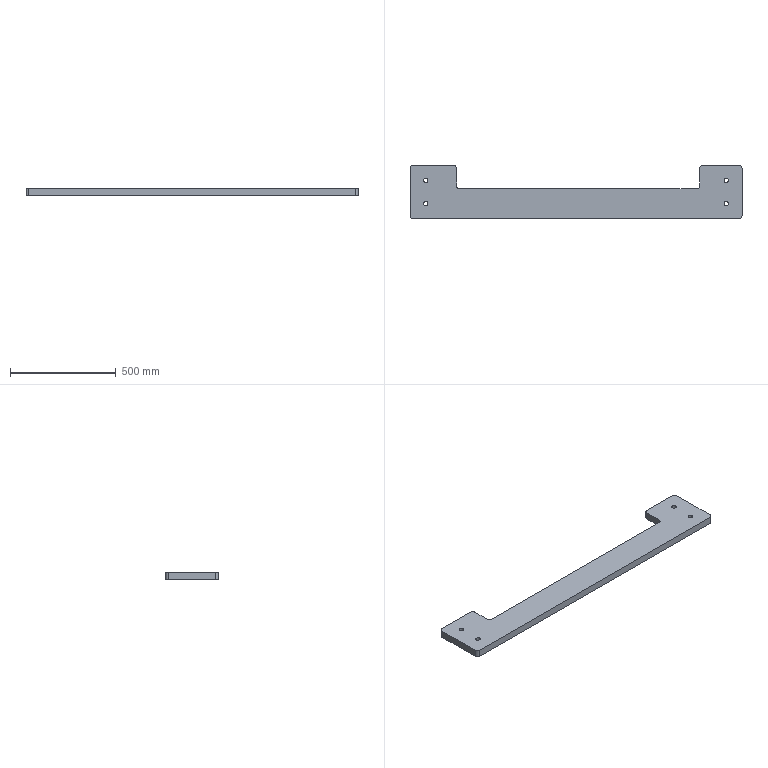Part | SolidWorks | features SavedExtBody 1 | 1 solid | 26 faces | box 1570 x 250 x 35 mm | volume 9261323 mm3 | cylinder 16 | plane 10 | commonest cylinder face diameters 20 x8 25 x8
STEP:
#1=CARTESIAN_POINT('',(-720.,-55.,0.));
#2=VERTEX_POINT('',#1);
#3=CARTESIAN_POINT('',(-700.,-55.,0.));
#4=VERTEX_POINT('',#3);
#5=CARTESIAN_POINT('',(-710.,-55.,0.));
#6=DIRECTION('',(0.,0.,1.));
#7=DIRECTION('',(-1.,0.,0.));
#8=AXIS2_PLACEMENT_3D('',#5,#6,#7);
#9=CIRCLE('',#8,10.);
#10=EDGE_CURVE('',#2,#4,#9,.T.);
#11=ORIENTED_EDGE('',*,*,#10,.F.);
#12=CARTESIAN_POINT('',(-720.,-55.,35.));
#13=VERTEX_POINT('',#12);
#14=CARTESIAN_POINT('',(-720.,-55.,-0.001));
#15=DIRECTION('',(0.,0.,1.));
#16=VECTOR('',#15,1000.);
#17=LINE('',#14,#16);
#18=EDGE_CURVE('',#2,#13,#17,.T.);
#19=ORIENTED_EDGE('',*,*,#18,.T.);
#20=CARTESIAN_POINT('',(-700.,-55.,35.));
#21=VERTEX_POINT('',#20);
#22=CARTESIAN_POINT('',(-710.,-55.,35.));
#23=DIRECTION('',(0.,0.,1.));
#24=DIRECTION('',(1.,0.,0.));
#25=AXIS2_PLACEMENT_3D('',#22,#23,#24);
#26=CIRCLE('',#25,10.);
#27=EDGE_CURVE('',#13,#21,#26,.T.);
#28=ORIENTED_EDGE('',*,*,#27,.T.);
#29=CARTESIAN_POINT('',(-700.,-55.,-0.001));
#30=DIRECTION('',(0.,0.,1.));
#31=VECTOR('',#30,1000.);
#32=LINE('',#29,#31);
#33=EDGE_CURVE('',#4,#21,#32,.T.);
#34=ORIENTED_EDGE('',*,*,#33,.F.);
#35=EDGE_LOOP('',(#11,#19,#28,#34));
#36=FACE_OUTER_BOUND('',#35,.T.);
#37=CARTESIAN_POINT('',(-710.,-55.,-0.001));
#38=DIRECTION('',(0.,0.,1.));
#39=DIRECTION('',(1.,0.,0.));
#40=AXIS2_PLACEMENT_3D('',#37,#38,#39);
#41=CYLINDRICAL_SURFACE('',#40,10.);
#42=ADVANCED_FACE('',(#36),#41,.F.);
#43=CARTESIAN_POINT('',(700.,55.,0.));
#44=VERTEX_POINT('',#43);
#45=CARTESIAN_POINT('',(720.,55.,0.));
#46=VERTEX_POINT('',#45);
#47=CARTESIAN_POINT('',(710.,55.,0.));
#48=DIRECTION('',(0.,0.,1.));
#49=DIRECTION('',(-1.,0.,0.));
#50=AXIS2_PLACEMENT_3D('',#47,#48,#49);
#51=CIRCLE('',#50,10.);
#52=EDGE_CURVE('',#44,#46,#51,.T.);
#53=ORIENTED_EDGE('',*,*,#52,.F.);
#54=CARTESIAN_POINT('',(700.,55.,35.));
#55=VERTEX_POINT('',#54);
#56=CARTESIAN_POINT('',(700.,55.,-0.001));
#57=DIRECTION('',(0.,0.,1.));
#58=VECTOR('',#57,1000.);
#59=LINE('',#56,#58);
#60=EDGE_CURVE('',#44,#55,#59,.T.);
#61=ORIENTED_EDGE('',*,*,#60,.T.);
#62=CARTESIAN_POINT('',(720.,55.,35.));
#63=VERTEX_POINT('',#62);
#64=CARTESIAN_POINT('',(710.,55.,35.));
#65=DIRECTION('',(0.,0.,1.));
#66=DIRECTION('',(1.,0.,0.));
#67=AXIS2_PLACEMENT_3D('',#64,#65,#66);
#68=CIRCLE('',#67,10.);
#69=EDGE_CURVE('',#55,#63,#68,.T.);
#70=ORIENTED_EDGE('',*,*,#69,.T.);
#71=CARTESIAN_POINT('',(720.,55.,-0.001));
#72=DIRECTION('',(0.,0.,1.));
#73=VECTOR('',#72,1000.);
#74=LINE('',#71,#73);
#75=EDGE_CURVE('',#46,#63,#74,.T.);
#76=ORIENTED_EDGE('',*,*,#75,.F.);
#77=EDGE_LOOP('',(#53,#61,#70,#76));
#78=FACE_OUTER_BOUND('',#77,.T.);
#79=CARTESIAN_POINT('',(710.,55.,-0.001));
#80=DIRECTION('',(0.,0.,1.));
#81=DIRECTION('',(1.,0.,0.));
#82=AXIS2_PLACEMENT_3D('',#79,#80,#81);
#83=CYLINDRICAL_SURFACE('',#82,10.);
#84=ADVANCED_FACE('',(#78),#83,.F.);
#85=CARTESIAN_POINT('',(700.,-55.,0.));
#86=VERTEX_POINT('',#85);
#87=CARTESIAN_POINT('',(720.,-55.,0.));
#88=VERTEX_POINT('',#87);
#89=CARTESIAN_POINT('',(710.,-55.,0.));
#90=DIRECTION('',(0.,0.,1.));
#91=DIRECTION('',(-1.,0.,0.));
#92=AXIS2_PLACEMENT_3D('',#89,#90,#91);
#93=CIRCLE('',#92,10.);
#94=EDGE_CURVE('',#86,#88,#93,.T.);
#95=ORIENTED_EDGE('',*,*,#94,.F.);
#96=CARTESIAN_POINT('',(700.,-55.,35.));
#97=VERTEX_POINT('',#96);
#98=CARTESIAN_POINT('',(700.,-55.,-0.001));
#99=DIRECTION('',(0.,0.,1.));
#100=VECTOR('',#99,1000.);
#101=LINE('',#98,#100);
#102=EDGE_CURVE('',#86,#97,#101,.T.);
#103=ORIENTED_EDGE('',*,*,#102,.T.);
#104=CARTESIAN_POINT('',(720.,-55.,35.));
#105=VERTEX_POINT('',#104);
#106=CARTESIAN_POINT('',(710.,-55.,35.));
#107=DIRECTION('',(0.,0.,1.));
#108=DIRECTION('',(1.,0.,0.));
#109=AXIS2_PLACEMENT_3D('',#106,#107,#108);
#110=CIRCLE('',#109,10.);
#111=EDGE_CURVE('',#97,#105,#110,.T.);
#112=ORIENTED_EDGE('',*,*,#111,.T.);
#113=CARTESIAN_POINT('',(720.,-55.,-0.001));
#114=DIRECTION('',(0.,0.,1.));
#115=VECTOR('',#114,1000.);
#116=LINE('',#113,#115);
#117=EDGE_CURVE('',#88,#105,#116,.T.);
#118=ORIENTED_EDGE('',*,*,#117,.F.);
#119=EDGE_LOOP('',(#95,#103,#112,#118));
#120=FACE_OUTER_BOUND('',#119,.T.);
#121=CARTESIAN_POINT('',(710.,-55.,-0.001));
#122=DIRECTION('',(0.,0.,1.));
#123=DIRECTION('',(1.,0.,0.));
#124=AXIS2_PLACEMENT_3D('',#121,#122,#123);
#125=CYLINDRICAL_SURFACE('',#124,10.);
#126=ADVANCED_FACE('',(#120),#125,.F.);
#127=CARTESIAN_POINT('',(-720.,55.,0.));
#128=VERTEX_POINT('',#127);
#129=CARTESIAN_POINT('',(-700.,55.,0.));
#130=VERTEX_POINT('',#129);
#131=CARTESIAN_POINT('',(-710.,55.,0.));
#132=DIRECTION('',(0.,0.,1.));
#133=DIRECTION('',(-1.,0.,0.));
#134=AXIS2_PLACEMENT_3D('',#131,#132,#133);
#135=CIRCLE('',#134,10.);
#136=EDGE_CURVE('',#128,#130,#135,.T.);
#137=ORIENTED_EDGE('',*,*,#136,.F.);
#138=CARTESIAN_POINT('',(-720.,55.,35.));
#139=VERTEX_POINT('',#138);
#140=CARTESIAN_POINT('',(-720.,55.,-0.001));
#141=DIRECTION('',(0.,0.,1.));
#142=VECTOR('',#141,1000.);
#143=LINE('',#140,#142);
#144=EDGE_CURVE('',#128,#139,#143,.T.);
#145=ORIENTED_EDGE('',*,*,#144,.T.);
#146=CARTESIAN_POINT('',(-700.,55.,35.));
#147=VERTEX_POINT('',#146);
#148=CARTESIAN_POINT('',(-710.,55.,35.));
#149=DIRECTION('',(0.,0.,1.));
#150=DIRECTION('',(1.,0.,0.));
#151=AXIS2_PLACEMENT_3D('',#148,#149,#150);
#152=CIRCLE('',#151,10.);
#153=EDGE_CURVE('',#139,#147,#152,.T.);
#154=ORIENTED_EDGE('',*,*,#153,.T.);
#155=CARTESIAN_POINT('',(-700.,55.,-0.001));
#156=DIRECTION('',(0.,0.,1.));
#157=VECTOR('',#156,1000.);
#158=LINE('',#155,#157);
#159=EDGE_CURVE('',#130,#147,#158,.T.);
#160=ORIENTED_EDGE('',*,*,#159,.F.);
#161=EDGE_LOOP('',(#137,#145,#154,#160));
#162=FACE_OUTER_BOUND('',#161,.T.);
#163=CARTESIAN_POINT('',(-710.,55.,-0.001));
#164=DIRECTION('',(0.,0.,1.));
#165=DIRECTION('',(1.,0.,0.));
#166=AXIS2_PLACEMENT_3D('',#163,#164,#165);
#167=CYLINDRICAL_SURFACE('',#166,10.);
#168=ADVANCED_FACE('',(#162),#167,.F.);
#169=CARTESIAN_POINT('',(772.5,125.,0.));
#170=VERTEX_POINT('',#169);
#171=CARTESIAN_POINT('',(597.5,125.,0.));
#172=VERTEX_POINT('',#171);
#173=CARTESIAN_POINT('',(-785.,125.,0.));
#174=DIRECTION('',(-1.,0.,0.));
#175=VECTOR('',#174,1000.);
#176=LINE('',#173,#175);
#177=EDGE_CURVE('',#170,#172,#176,.T.);
#178=ORIENTED_EDGE('',*,*,#177,.T.);
#179=CARTESIAN_POINT('',(597.5,125.,35.));
#180=VERTEX_POINT('',#179);
#181=CARTESIAN_POINT('',(597.5,125.,35.));
#182=DIRECTION('',(0.,0.,1.));
#183=VECTOR('',#182,1000.);
#184=LINE('',#181,#183);
#185=EDGE_CURVE('',#172,#180,#184,.T.);
#186=ORIENTED_EDGE('',*,*,#185,.T.);
#187=CARTESIAN_POINT('',(772.5,125.,35.));
#188=VERTEX_POINT('',#187);
#189=CARTESIAN_POINT('',(-785.,125.,35.));
#190=DIRECTION('',(-1.,0.,0.));
#191=VECTOR('',#190,1000.);
#192=LINE('',#189,#191);
#193=EDGE_CURVE('',#188,#180,#192,.T.);
#194=ORIENTED_EDGE('',*,*,#193,.F.);
#195=CARTESIAN_POINT('',(772.5,125.,35.));
#196=DIRECTION('',(0.,0.,-1.));
#197=VECTOR('',#196,1000.);
#198=LINE('',#195,#197);
#199=EDGE_CURVE('',#188,#170,#198,.T.);
#200=ORIENTED_EDGE('',*,*,#199,.T.);
#201=EDGE_LOOP('',(#178,#186,#194,#200));
#202=FACE_OUTER_BOUND('',#201,.T.);
#203=CARTESIAN_POINT('',(-785.,125.,35.));
#204=DIRECTION('',(0.,-1.,0.));
#205=DIRECTION('',(0.,0.,-1.));
#206=AXIS2_PLACEMENT_3D('',#203,#204,#205);
#207=PLANE('',#206);
#208=ADVANCED_FACE('',(#202),#207,.F.);
#209=CARTESIAN_POINT('',(785.,-112.5,0.));
#210=VERTEX_POINT('',#209);
#211=CARTESIAN_POINT('',(785.,112.5,0.));
#212=VERTEX_POINT('',#211);
#213=CARTESIAN_POINT('',(785.,-125.,0.));
#214=DIRECTION('',(0.,1.,0.));
#215=VECTOR('',#214,1000.);
#216=LINE('',#213,#215);
#217=EDGE_CURVE('',#210,#212,#216,.T.);
#218=ORIENTED_EDGE('',*,*,#217,.T.);
#219=CARTESIAN_POINT('',(785.,112.5,35.));
#220=VERTEX_POINT('',#219);
#221=CARTESIAN_POINT('',(785.,112.5,35.));
#222=DIRECTION('',(0.,0.,1.));
#223=VECTOR('',#222,1000.);
#224=LINE('',#221,#223);
#225=EDGE_CURVE('',#212,#220,#224,.T.);
#226=ORIENTED_EDGE('',*,*,#225,.T.);
#227=CARTESIAN_POINT('',(785.,-112.5,35.));
#228=VERTEX_POINT('',#227);
#229=CARTESIAN_POINT('',(785.,-125.,35.));
#230=DIRECTION('',(0.,1.,0.));
#231=VECTOR('',#230,1000.);
#232=LINE('',#229,#231);
#233=EDGE_CURVE('',#228,#220,#232,.T.);
#234=ORIENTED_EDGE('',*,*,#233,.F.);
#235=CARTESIAN_POINT('',(785.,-112.5,35.));
#236=DIRECTION('',(0.,0.,-1.));
#237=VECTOR('',#236,1000.);
#238=LINE('',#235,#237);
#239=EDGE_CURVE('',#228,#210,#238,.T.);
#240=ORIENTED_EDGE('',*,*,#239,.T.);
#241=EDGE_LOOP('',(#218,#226,#234,#240));
#242=FACE_OUTER_BOUND('',#241,.T.);
#243=CARTESIAN_POINT('',(785.,-125.,35.));
#244=DIRECTION('',(-1.,0.,0.));
#245=DIRECTION('',(0.,0.,1.));
#246=AXIS2_PLACEMENT_3D('',#243,#244,#245);
#247=PLANE('',#246);
#248=ADVANCED_FACE('',(#242),#247,.F.);
#249=CARTESIAN_POINT('',(-577.5,125.,35.));
#250=VERTEX_POINT('',#249);
#251=CARTESIAN_POINT('',(-772.5,125.,35.));
#252=VERTEX_POINT('',#251);
#253=CARTESIAN_POINT('',(-785.,125.,35.));
#254=DIRECTION('',(-1.,0.,0.));
#255=VECTOR('',#254,1000.);
#256=LINE('',#253,#255);
#257=EDGE_CURVE('',#250,#252,#256,.T.);
#258=ORIENTED_EDGE('',*,*,#257,.F.);
#259=CARTESIAN_POINT('',(-577.5,125.,0.));
#260=VERTEX_POINT('',#259);
#261=CARTESIAN_POINT('',(-577.5,125.,35.));
#262=DIRECTION('',(0.,0.,-1.));
#263=VECTOR('',#262,1000.);
#264=LINE('',#261,#263);
#265=EDGE_CURVE('',#250,#260,#264,.T.);
#266=ORIENTED_EDGE('',*,*,#265,.T.);
#267=CARTESIAN_POINT('',(-772.5,125.,0.));
#268=VERTEX_POINT('',#267);
#269=CARTESIAN_POINT('',(-785.,125.,0.));
#270=DIRECTION('',(-1.,0.,0.));
#271=VECTOR('',#270,1000.);
#272=LINE('',#269,#271);
#273=EDGE_CURVE('',#260,#268,#272,.T.);
#274=ORIENTED_EDGE('',*,*,#273,.T.);
#275=CARTESIAN_POINT('',(-772.5,125.,35.));
#276=DIRECTION('',(0.,0.,1.));
#277=VECTOR('',#276,1000.);
#278=LINE('',#275,#277);
#279=EDGE_CURVE('',#268,#252,#278,.T.);
#280=ORIENTED_EDGE('',*,*,#279,.T.);
#281=EDGE_LOOP('',(#258,#266,#274,#280));
#282=FACE_OUTER_BOUND('',#281,.T.);
#283=CARTESIAN_POINT('',(-785.,125.,35.));
#284=DIRECTION('',(0.,-1.,0.));
#285=DIRECTION('',(0.,0.,-1.));
#286=AXIS2_PLACEMENT_3D('',#283,#284,#285);
#287=PLANE('',#286);
#288=ADVANCED_FACE('',(#282),#287,.F.);
#289=CARTESIAN_POINT('',(-785.,112.5,0.));
#290=VERTEX_POINT('',#289);
#291=CARTESIAN_POINT('',(-785.,-112.5,0.));
#292=VERTEX_POINT('',#291);
#293=CARTESIAN_POINT('',(-785.,-125.,0.));
#294=DIRECTION('',(0.,-1.,0.));
#295=VECTOR('',#294,1000.);
#296=LINE('',#293,#295);
#297=EDGE_CURVE('',#290,#292,#296,.T.);
#298=ORIENTED_EDGE('',*,*,#297,.T.);
#299=CARTESIAN_POINT('',(-785.,-112.5,35.));
#300=VERTEX_POINT('',#299);
#301=CARTESIAN_POINT('',(-785.,-112.5,35.));
#302=DIRECTION('',(0.,0.,1.));
#303=VECTOR('',#302,1000.);
#304=LINE('',#301,#303);
#305=EDGE_CURVE('',#292,#300,#304,.T.);
#306=ORIENTED_EDGE('',*,*,#305,.T.);
#307=CARTESIAN_POINT('',(-785.,112.5,35.));
#308=VERTEX_POINT('',#307);
#309=CARTESIAN_POINT('',(-785.,-125.,35.));
#310=DIRECTION('',(0.,-1.,0.));
#311=VECTOR('',#310,1000.);
#312=LINE('',#309,#311);
#313=EDGE_CURVE('',#308,#300,#312,.T.);
#314=ORIENTED_EDGE('',*,*,#313,.F.);
#315=CARTESIAN_POINT('',(-785.,112.5,35.));
#316=DIRECTION('',(0.,0.,-1.));
#317=VECTOR('',#316,1000.);
#318=LINE('',#315,#317);
#319=EDGE_CURVE('',#308,#290,#318,.T.);
#320=ORIENTED_EDGE('',*,*,#319,.T.);
#321=EDGE_LOOP('',(#298,#306,#314,#320));
#322=FACE_OUTER_BOUND('',#321,.T.);
#323=CARTESIAN_POINT('',(-785.,-125.,35.));
#324=DIRECTION('',(1.,0.,0.));
#325=DIRECTION('',(0.,0.,-1.));
#326=AXIS2_PLACEMENT_3D('',#323,#324,#325);
#327=PLANE('',#326);
#328=ADVANCED_FACE('',(#322),#327,.F.);
#329=CARTESIAN_POINT('',(-772.5,-125.,0.));
#330=VERTEX_POINT('',#329);
#331=CARTESIAN_POINT('',(772.5,-125.,0.));
#332=VERTEX_POINT('',#331);
#333=CARTESIAN_POINT('',(-785.,-125.,0.));
#334=DIRECTION('',(1.,0.,0.));
#335=VECTOR('',#334,1000.);
#336=LINE('',#333,#335);
#337=EDGE_CURVE('',#330,#332,#336,.T.);
#338=ORIENTED_EDGE('',*,*,#337,.T.);
#339=CARTESIAN_POINT('',(772.5,-125.,35.));
#340=VERTEX_POINT('',#339);
#341=CARTESIAN_POINT('',(772.5,-125.,35.));
#342=DIRECTION('',(0.,0.,1.));
#343=VECTOR('',#342,1000.);
#344=LINE('',#341,#343);
#345=EDGE_CURVE('',#332,#340,#344,.T.);
#346=ORIENTED_EDGE('',*,*,#345,.T.);
#347=CARTESIAN_POINT('',(-772.5,-125.,35.));
#348=VERTEX_POINT('',#347);
#349=CARTESIAN_POINT('',(-785.,-125.,35.));
#350=DIRECTION('',(1.,0.,0.));
#351=VECTOR('',#350,1000.);
#352=LINE('',#349,#351);
#353=EDGE_CURVE('',#348,#340,#352,.T.);
#354=ORIENTED_EDGE('',*,*,#353,.F.);
#355=CARTESIAN_POINT('',(-772.5,-125.,35.));
#356=DIRECTION('',(0.,0.,-1.));
#357=VECTOR('',#356,1000.);
#358=LINE('',#355,#357);
#359=EDGE_CURVE('',#348,#330,#358,.T.);
#360=ORIENTED_EDGE('',*,*,#359,.T.);
#361=EDGE_LOOP('',(#338,#346,#354,#360));
#362=FACE_OUTER_BOUND('',#361,.T.);
#363=CARTESIAN_POINT('',(-785.,-125.,35.));
#364=DIRECTION('',(0.,1.,0.));
#365=DIRECTION('',(0.,0.,1.));
#366=AXIS2_PLACEMENT_3D('',#363,#364,#365);
#367=PLANE('',#366);
#368=ADVANCED_FACE('',(#362),#367,.F.);
#369=CARTESIAN_POINT('',(-710.,-55.,35.));
#370=DIRECTION('',(0.,0.,1.));
#371=DIRECTION('',(1.,0.,0.));
#372=AXIS2_PLACEMENT_3D('',#369,#370,#371);
#373=CIRCLE('',#372,10.);
#374=EDGE_CURVE('',#21,#13,#373,.T.);
#375=ORIENTED_EDGE('',*,*,#374,.F.);
#376=ORIENTED_EDGE('',*,*,#27,.F.);
#377=EDGE_LOOP('',(#375,#376));
#378=FACE_BOUND('',#377,.T.);
#379=CARTESIAN_POINT('',(710.,55.,35.));
#380=DIRECTION('',(0.,0.,1.));
#381=DIRECTION('',(1.,0.,0.));
#382=AXIS2_PLACEMENT_3D('',#379,#380,#381);
#383=CIRCLE('',#382,10.);
#384=EDGE_CURVE('',#63,#55,#383,.T.);
#385=ORIENTED_EDGE('',*,*,#384,.F.);
#386=ORIENTED_EDGE('',*,*,#69,.F.);
#387=EDGE_LOOP('',(#385,#386));
#388=FACE_BOUND('',#387,.T.);
#389=CARTESIAN_POINT('',(710.,-55.,35.));
#390=DIRECTION('',(0.,0.,1.));
#391=DIRECTION('',(1.,0.,0.));
#392=AXIS2_PLACEMENT_3D('',#389,#390,#391);
#393=CIRCLE('',#392,10.);
#394=EDGE_CURVE('',#105,#97,#393,.T.);
#395=ORIENTED_EDGE('',*,*,#394,.F.);
#396=ORIENTED_EDGE('',*,*,#111,.F.);
#397=EDGE_LOOP('',(#395,#396));
#398=FACE_BOUND('',#397,.T.);
#399=CARTESIAN_POINT('',(-710.,55.,35.));
#400=DIRECTION('',(0.,0.,1.));
#401=DIRECTION('',(1.,0.,0.));
#402=AXIS2_PLACEMENT_3D('',#399,#400,#401);
#403=CIRCLE('',#402,10.);
#404=EDGE_CURVE('',#147,#139,#403,.T.);
#405=ORIENTED_EDGE('',*,*,#404,.F.);
#406=ORIENTED_EDGE('',*,*,#153,.F.);
#407=EDGE_LOOP('',(#405,#406));
#408=FACE_BOUND('',#407,.T.);
#409=CARTESIAN_POINT('',(-565.,112.5,35.));
#410=VERTEX_POINT('',#409);
#411=CARTESIAN_POINT('',(-565.,27.5,35.));
#412=VERTEX_POINT('',#411);
#413=CARTESIAN_POINT('',(-565.,125.,35.));
#414=DIRECTION('',(0.,-1.,0.));
#415=VECTOR('',#414,1000.);
#416=LINE('',#413,#415);
#417=EDGE_CURVE('',#410,#412,#416,.T.);
#418=ORIENTED_EDGE('',*,*,#417,.F.);
#419=CARTESIAN_POINT('',(-577.5,112.5,35.));
#420=DIRECTION('',(0.,0.,1.));
#421=DIRECTION('',(-1.,0.,0.));
#422=AXIS2_PLACEMENT_3D('',#419,#420,#421);
#423=CIRCLE('',#422,12.5);
#424=EDGE_CURVE('',#410,#250,#423,.T.);
#425=ORIENTED_EDGE('',*,*,#424,.T.);
#426=ORIENTED_EDGE('',*,*,#257,.T.);
#427=CARTESIAN_POINT('',(-772.5,112.5,35.));
#428=DIRECTION('',(0.,0.,1.));
#429=DIRECTION('',(-1.,0.,0.));
#430=AXIS2_PLACEMENT_3D('',#427,#428,#429);
#431=CIRCLE('',#430,12.5);
#432=EDGE_CURVE('',#252,#308,#431,.T.);
#433=ORIENTED_EDGE('',*,*,#432,.T.);
#434=ORIENTED_EDGE('',*,*,#313,.T.);
#435=CARTESIAN_POINT('',(-772.5,-112.5,35.));
#436=DIRECTION('',(0.,0.,1.));
#437=DIRECTION('',(-1.,0.,0.));
#438=AXIS2_PLACEMENT_3D('',#435,#436,#437);
#439=CIRCLE('',#438,12.5);
#440=EDGE_CURVE('',#300,#348,#439,.T.);
#441=ORIENTED_EDGE('',*,*,#440,.T.);
#442=ORIENTED_EDGE('',*,*,#353,.T.);
#443=CARTESIAN_POINT('',(772.5,-112.5,35.));
#444=DIRECTION('',(0.,0.,1.));
#445=DIRECTION('',(-1.,0.,0.));
#446=AXIS2_PLACEMENT_3D('',#443,#444,#445);
#447=CIRCLE('',#446,12.5);
#448=EDGE_CURVE('',#340,#228,#447,.T.);
#449=ORIENTED_EDGE('',*,*,#448,.T.);
#450=ORIENTED_EDGE('',*,*,#233,.T.);
#451=CARTESIAN_POINT('',(772.5,112.5,35.));
#452=DIRECTION('',(0.,0.,1.));
#453=DIRECTION('',(-1.,0.,0.));
#454=AXIS2_PLACEMENT_3D('',#451,#452,#453);
#455=CIRCLE('',#454,12.5);
#456=EDGE_CURVE('',#220,#188,#455,.T.);
#457=ORIENTED_EDGE('',*,*,#456,.T.);
#458=ORIENTED_EDGE('',*,*,#193,.T.);
#459=CARTESIAN_POINT('',(585.,112.5,35.));
#460=VERTEX_POINT('',#459);
#461=CARTESIAN_POINT('',(597.5,112.5,35.));
#462=DIRECTION('',(0.,0.,1.));
#463=DIRECTION('',(-1.,0.,0.));
#464=AXIS2_PLACEMENT_3D('',#461,#462,#463);
#465=CIRCLE('',#464,12.5);
#466=EDGE_CURVE('',#180,#460,#465,.T.);
#467=ORIENTED_EDGE('',*,*,#466,.T.);
#468=CARTESIAN_POINT('',(585.,27.5,35.));
#469=VERTEX_POINT('',#468);
#470=CARTESIAN_POINT('',(585.,15.,35.));
#471=DIRECTION('',(0.,1.,0.));
#472=VECTOR('',#471,1000.);
#473=LINE('',#470,#472);
#474=EDGE_CURVE('',#469,#460,#473,.T.);
#475=ORIENTED_EDGE('',*,*,#474,.F.);
#476=CARTESIAN_POINT('',(572.5,15.,35.));
#477=VERTEX_POINT('',#476);
#478=CARTESIAN_POINT('',(572.5,27.5,35.));
#479=DIRECTION('',(0.,0.,-1.));
#480=DIRECTION('',(-1.,0.,0.));
#481=AXIS2_PLACEMENT_3D('',#478,#479,#480);
#482=CIRCLE('',#481,12.5);
#483=EDGE_CURVE('',#469,#477,#482,.T.);
#484=ORIENTED_EDGE('',*,*,#483,.T.);
#485=CARTESIAN_POINT('',(-552.5,15.,35.));
#486=VERTEX_POINT('',#485);
#487=CARTESIAN_POINT('',(-565.,15.,35.));
#488=DIRECTION('',(1.,0.,0.));
#489=VECTOR('',#488,1000.);
#490=LINE('',#487,#489);
#491=EDGE_CURVE('',#486,#477,#490,.T.);
#492=ORIENTED_EDGE('',*,*,#491,.F.);
#493=CARTESIAN_POINT('',(-552.5,27.5,35.));
#494=DIRECTION('',(0.,0.,-1.));
#495=DIRECTION('',(-1.,0.,0.));
#496=AXIS2_PLACEMENT_3D('',#493,#494,#495);
#497=CIRCLE('',#496,12.5);
#498=EDGE_CURVE('',#486,#412,#497,.T.);
#499=ORIENTED_EDGE('',*,*,#498,.T.);
#500=EDGE_LOOP('',(#418,#425,#426,#433,#434,#441,#442,#449,#450,#457,#458,#467,#475,#484,#492,#499));
#501=FACE_OUTER_BOUND('',#500,.T.);
#502=CARTESIAN_POINT('',(0.,0.,35.));
#503=DIRECTION('',(0.,0.,-1.));
#504=DIRECTION('',(-1.,0.,0.));
#505=AXIS2_PLACEMENT_3D('',#502,#503,#504);
#506=PLANE('',#505);
#507=ADVANCED_FACE('',(#378,#388,#398,#408,#501),#506,.F.);
#508=CARTESIAN_POINT('',(-710.,-55.,0.));
#509=DIRECTION('',(0.,0.,1.));
#510=DIRECTION('',(-1.,0.,0.));
#511=AXIS2_PLACEMENT_3D('',#508,#509,#510);
#512=CIRCLE('',#511,10.);
#513=EDGE_CURVE('',#4,#2,#512,.T.);
#514=ORIENTED_EDGE('',*,*,#513,.T.);
#515=ORIENTED_EDGE('',*,*,#10,.T.);
#516=EDGE_LOOP('',(#514,#515));
#517=FACE_BOUND('',#516,.T.);
#518=CARTESIAN_POINT('',(710.,55.,0.));
#519=DIRECTION('',(0.,0.,1.));
#520=DIRECTION('',(-1.,0.,0.));
#521=AXIS2_PLACEMENT_3D('',#518,#519,#520);
#522=CIRCLE('',#521,10.);
#523=EDGE_CURVE('',#46,#44,#522,.T.);
#524=ORIENTED_EDGE('',*,*,#523,.T.);
#525=ORIENTED_EDGE('',*,*,#52,.T.);
#526=EDGE_LOOP('',(#524,#525));
#527=FACE_BOUND('',#526,.T.);
#528=CARTESIAN_POINT('',(710.,-55.,0.));
#529=DIRECTION('',(0.,0.,1.));
#530=DIRECTION('',(-1.,0.,0.));
#531=AXIS2_PLACEMENT_3D('',#528,#529,#530);
#532=CIRCLE('',#531,10.);
#533=EDGE_CURVE('',#88,#86,#532,.T.);
#534=ORIENTED_EDGE('',*,*,#533,.T.);
#535=ORIENTED_EDGE('',*,*,#94,.T.);
#536=EDGE_LOOP('',(#534,#535));
#537=FACE_BOUND('',#536,.T.);
#538=CARTESIAN_POINT('',(-710.,55.,0.));
#539=DIRECTION('',(0.,0.,1.));
#540=DIRECTION('',(-1.,0.,0.));
#541=AXIS2_PLACEMENT_3D('',#538,#539,#540);
#542=CIRCLE('',#541,10.);
#543=EDGE_CURVE('',#130,#128,#542,.T.);
#544=ORIENTED_EDGE('',*,*,#543,.T.);
#545=ORIENTED_EDGE('',*,*,#136,.T.);
#546=EDGE_LOOP('',(#544,#545));
#547=FACE_BOUND('',#546,.T.);
#548=ORIENTED_EDGE('',*,*,#273,.F.);
#549=CARTESIAN_POINT('',(-565.,112.5,0.));
#550=VERTEX_POINT('',#549);
#551=CARTESIAN_POINT('',(-577.5,112.5,0.));
#552=DIRECTION('',(0.,0.,-1.));
#553=DIRECTION('',(-1.,0.,0.));
#554=AXIS2_PLACEMENT_3D('',#551,#552,#553);
#555=CIRCLE('',#554,12.5);
#556=EDGE_CURVE('',#260,#550,#555,.T.);
#557=ORIENTED_EDGE('',*,*,#556,.T.);
#558=CARTESIAN_POINT('',(-565.,27.5,0.));
#559=VERTEX_POINT('',#558);
#560=CARTESIAN_POINT('',(-565.,125.,0.));
#561=DIRECTION('',(0.,-1.,0.));
#562=VECTOR('',#561,1000.);
#563=LINE('',#560,#562);
#564=EDGE_CURVE('',#550,#559,#563,.T.);
#565=ORIENTED_EDGE('',*,*,#564,.T.);
#566=CARTESIAN_POINT('',(-552.5,15.,0.));
#567=VERTEX_POINT('',#566);
#568=CARTESIAN_POINT('',(-552.5,27.5,0.));
#569=DIRECTION('',(0.,0.,1.));
#570=DIRECTION('',(-1.,0.,0.));
#571=AXIS2_PLACEMENT_3D('',#568,#569,#570);
#572=CIRCLE('',#571,12.5);
#573=EDGE_CURVE('',#559,#567,#572,.T.);
#574=ORIENTED_EDGE('',*,*,#573,.T.);
#575=CARTESIAN_POINT('',(572.5,15.,0.));
#576=VERTEX_POINT('',#575);
#577=CARTESIAN_POINT('',(-565.,15.,0.));
#578=DIRECTION('',(1.,0.,0.));
#579=VECTOR('',#578,1000.);
#580=LINE('',#577,#579);
#581=EDGE_CURVE('',#567,#576,#580,.T.);
#582=ORIENTED_EDGE('',*,*,#581,.T.);
#583=CARTESIAN_POINT('',(585.,27.5,0.));
#584=VERTEX_POINT('',#583);
#585=CARTESIAN_POINT('',(572.5,27.5,0.));
#586=DIRECTION('',(0.,0.,1.));
#587=DIRECTION('',(-1.,0.,0.));
#588=AXIS2_PLACEMENT_3D('',#585,#586,#587);
#589=CIRCLE('',#588,12.5);
#590=EDGE_CURVE('',#576,#584,#589,.T.);
#591=ORIENTED_EDGE('',*,*,#590,.T.);
#592=CARTESIAN_POINT('',(585.,112.5,0.));
#593=VERTEX_POINT('',#592);
#594=CARTESIAN_POINT('',(585.,15.,0.));
#595=DIRECTION('',(0.,1.,0.));
#596=VECTOR('',#595,1000.);
#597=LINE('',#594,#596);
#598=EDGE_CURVE('',#584,#593,#597,.T.);
#599=ORIENTED_EDGE('',*,*,#598,.T.);
#600=CARTESIAN_POINT('',(597.5,112.5,0.));
#601=DIRECTION('',(0.,0.,-1.));
#602=DIRECTION('',(-1.,0.,0.));
#603=AXIS2_PLACEMENT_3D('',#600,#601,#602);
#604=CIRCLE('',#603,12.5);
#605=EDGE_CURVE('',#593,#172,#604,.T.);
#606=ORIENTED_EDGE('',*,*,#605,.T.);
#607=ORIENTED_EDGE('',*,*,#177,.F.);
#608=CARTESIAN_POINT('',(772.5,112.5,0.));
#609=DIRECTION('',(0.,0.,-1.));
#610=DIRECTION('',(-1.,0.,0.));
#611=AXIS2_PLACEMENT_3D('',#608,#609,#610);
#612=CIRCLE('',#611,12.5);
#613=EDGE_CURVE('',#170,#212,#612,.T.);
#614=ORIENTED_EDGE('',*,*,#613,.T.);
#615=ORIENTED_EDGE('',*,*,#217,.F.);
#616=CARTESIAN_POINT('',(772.5,-112.5,0.));
#617=DIRECTION('',(0.,0.,-1.));
#618=DIRECTION('',(-1.,0.,0.));
#619=AXIS2_PLACEMENT_3D('',#616,#617,#618);
#620=CIRCLE('',#619,12.5);
#621=EDGE_CURVE('',#210,#332,#620,.T.);
#622=ORIENTED_EDGE('',*,*,#621,.T.);
#623=ORIENTED_EDGE('',*,*,#337,.F.);
#624=CARTESIAN_POINT('',(-772.5,-112.5,0.));
#625=DIRECTION('',(0.,0.,-1.));
#626=DIRECTION('',(-1.,0.,0.));
#627=AXIS2_PLACEMENT_3D('',#624,#625,#626);
#628=CIRCLE('',#627,12.5);
#629=EDGE_CURVE('',#330,#292,#628,.T.);
#630=ORIENTED_EDGE('',*,*,#629,.T.);
#631=ORIENTED_EDGE('',*,*,#297,.F.);
#632=CARTESIAN_POINT('',(-772.5,112.5,0.));
#633=DIRECTION('',(0.,0.,-1.));
#634=DIRECTION('',(-1.,0.,0.));
#635=AXIS2_PLACEMENT_3D('',#632,#633,#634);
#636=CIRCLE('',#635,12.5);
#637=EDGE_CURVE('',#290,#268,#636,.T.);
#638=ORIENTED_EDGE('',*,*,#637,.T.);
#639=EDGE_LOOP('',(#548,#557,#565,#574,#582,#591,#599,#606,#607,#614,#615,#622,#623,#630,#631,#638));
#640=FACE_OUTER_BOUND('',#639,.T.);
#641=CARTESIAN_POINT('',(0.,0.,0.));
#642=DIRECTION('',(0.,0.,-1.));
#643=DIRECTION('',(-1.,0.,0.));
#644=AXIS2_PLACEMENT_3D('',#641,#642,#643);
#645=PLANE('',#644);
#646=ADVANCED_FACE('',(#517,#527,#537,#547,#640),#645,.T.);
#647=ORIENTED_EDGE('',*,*,#598,.F.);
#648=CARTESIAN_POINT('',(585.,27.5,35.));
#649=DIRECTION('',(0.,0.,1.));
#650=VECTOR('',#649,1000.);
#651=LINE('',#648,#650);
#652=EDGE_CURVE('',#584,#469,#651,.T.);
#653=ORIENTED_EDGE('',*,*,#652,.T.);
#654=ORIENTED_EDGE('',*,*,#474,.T.);
#655=CARTESIAN_POINT('',(585.,112.5,-0.001));
#656=DIRECTION('',(0.,0.,-1.));
#657=VECTOR('',#656,1000.);
#658=LINE('',#655,#657);
#659=EDGE_CURVE('',#460,#593,#658,.T.);
#660=ORIENTED_EDGE('',*,*,#659,.T.);
#661=EDGE_LOOP('',(#647,#653,#654,#660));
#662=FACE_OUTER_BOUND('',#661,.T.);
#663=CARTESIAN_POINT('',(585.,15.,-0.001));
#664=DIRECTION('',(1.,0.,0.));
#665=DIRECTION('',(0.,1.,0.));
#666=AXIS2_PLACEMENT_3D('',#663,#664,#665);
#667=PLANE('',#666);
#668=ADVANCED_FACE('',(#662),#667,.F.);
#669=ORIENTED_EDGE('',*,*,#581,.F.);
#670=CARTESIAN_POINT('',(-552.5,15.,35.));
#671=DIRECTION('',(0.,0.,1.));
#672=VECTOR('',#671,1000.);
#673=LINE('',#670,#672);
#674=EDGE_CURVE('',#567,#486,#673,.T.);
#675=ORIENTED_EDGE('',*,*,#674,.T.);
#676=ORIENTED_EDGE('',*,*,#491,.T.);
#677=CARTESIAN_POINT('',(572.5,15.,0.));
#678=DIRECTION('',(0.,0.,-1.));
#679=VECTOR('',#678,1000.);
#680=LINE('',#677,#679);
#681=EDGE_CURVE('',#477,#576,#680,.T.);
#682=ORIENTED_EDGE('',*,*,#681,.T.);
#683=EDGE_LOOP('',(#669,#675,#676,#682));
#684=FACE_OUTER_BOUND('',#683,.T.);
#685=CARTESIAN_POINT('',(-565.,15.,-0.001));
#686=DIRECTION('',(0.,-1.,0.));
#687=DIRECTION('',(0.,0.,-1.));
#688=AXIS2_PLACEMENT_3D('',#685,#686,#687);
#689=PLANE('',#688);
#690=ADVANCED_FACE('',(#684),#689,.F.);
#691=ORIENTED_EDGE('',*,*,#417,.T.);
#692=CARTESIAN_POINT('',(-565.,27.5,0.));
#693=DIRECTION('',(0.,0.,-1.));
#694=VECTOR('',#693,1000.);
#695=LINE('',#692,#694);
#696=EDGE_CURVE('',#412,#559,#695,.T.);
#697=ORIENTED_EDGE('',*,*,#696,.T.);
#698=ORIENTED_EDGE('',*,*,#564,.F.);
#699=CARTESIAN_POINT('',(-565.,112.5,-0.001));
#700=DIRECTION('',(0.,0.,1.));
#701=VECTOR('',#700,1000.);
#702=LINE('',#699,#701);
#703=EDGE_CURVE('',#550,#410,#702,.T.);
#704=ORIENTED_EDGE('',*,*,#703,.T.);
#705=EDGE_LOOP('',(#691,#697,#698,#704));
#706=FACE_OUTER_BOUND('',#705,.T.);
#707=CARTESIAN_POINT('',(-565.,125.,-0.001));
#708=DIRECTION('',(-1.,0.,0.));
#709=DIRECTION('',(0.,0.,1.));
#710=AXIS2_PLACEMENT_3D('',#707,#708,#709);
#711=PLANE('',#710);
#712=ADVANCED_FACE('',(#706),#711,.F.);
#713=ORIENTED_EDGE('',*,*,#573,.F.);
#714=ORIENTED_EDGE('',*,*,#696,.F.);
#715=ORIENTED_EDGE('',*,*,#498,.F.);
#716=ORIENTED_EDGE('',*,*,#674,.F.);
#717=EDGE_LOOP('',(#713,#714,#715,#716));
#718=FACE_OUTER_BOUND('',#717,.T.);
#719=CARTESIAN_POINT('',(-552.5,27.5,-0.001));
#720=DIRECTION('',(0.,0.,-1.));
#721=DIRECTION('',(-1.,0.,0.));
#722=AXIS2_PLACEMENT_3D('',#719,#720,#721);
#723=CYLINDRICAL_SURFACE('',#722,12.5);
#724=ADVANCED_FACE('',(#718),#723,.F.);
#725=ORIENTED_EDGE('',*,*,#556,.F.);
#726=ORIENTED_EDGE('',*,*,#265,.F.);
#727=ORIENTED_EDGE('',*,*,#424,.F.);
#728=ORIENTED_EDGE('',*,*,#703,.F.);
#729=EDGE_LOOP('',(#725,#726,#727,#728));
#730=FACE_OUTER_BOUND('',#729,.T.);
#731=CARTESIAN_POINT('',(-577.5,112.5,-0.001));
#732=DIRECTION('',(0.,0.,1.));
#733=DIRECTION('',(1.,0.,0.));
#734=AXIS2_PLACEMENT_3D('',#731,#732,#733);
#735=CYLINDRICAL_SURFACE('',#734,12.5);
#736=ADVANCED_FACE('',(#730),#735,.T.);
#737=ORIENTED_EDGE('',*,*,#590,.F.);
#738=ORIENTED_EDGE('',*,*,#681,.F.);
#739=ORIENTED_EDGE('',*,*,#483,.F.);
#740=ORIENTED_EDGE('',*,*,#652,.F.);
#741=EDGE_LOOP('',(#737,#738,#739,#740));
#742=FACE_OUTER_BOUND('',#741,.T.);
#743=CARTESIAN_POINT('',(572.5,27.5,-0.001));
#744=DIRECTION('',(0.,0.,-1.));
#745=DIRECTION('',(-1.,0.,0.));
#746=AXIS2_PLACEMENT_3D('',#743,#744,#745);
#747=CYLINDRICAL_SURFACE('',#746,12.5);
#748=ADVANCED_FACE('',(#742),#747,.F.);
#749=ORIENTED_EDGE('',*,*,#605,.F.);
#750=ORIENTED_EDGE('',*,*,#659,.F.);
#751=ORIENTED_EDGE('',*,*,#466,.F.);
#752=ORIENTED_EDGE('',*,*,#185,.F.);
#753=EDGE_LOOP('',(#749,#750,#751,#752));
#754=FACE_OUTER_BOUND('',#753,.T.);
#755=CARTESIAN_POINT('',(597.5,112.5,35.));
#756=DIRECTION('',(0.,0.,1.));
#757=DIRECTION('',(1.,0.,0.));
#758=AXIS2_PLACEMENT_3D('',#755,#756,#757);
#759=CYLINDRICAL_SURFACE('',#758,12.5);
#760=ADVANCED_FACE('',(#754),#759,.T.);
#761=ORIENTED_EDGE('',*,*,#456,.F.);
#762=ORIENTED_EDGE('',*,*,#225,.F.);
#763=ORIENTED_EDGE('',*,*,#613,.F.);
#764=ORIENTED_EDGE('',*,*,#199,.F.);
#765=EDGE_LOOP('',(#761,#762,#763,#764));
#766=FACE_OUTER_BOUND('',#765,.T.);
#767=CARTESIAN_POINT('',(772.5,112.5,35.));
#768=DIRECTION('',(0.,0.,-1.));
#769=DIRECTION('',(-1.,0.,0.));
#770=AXIS2_PLACEMENT_3D('',#767,#768,#769);
#771=CYLINDRICAL_SURFACE('',#770,12.5);
#772=ADVANCED_FACE('',(#766),#771,.T.);
#773=ORIENTED_EDGE('',*,*,#448,.F.);
#774=ORIENTED_EDGE('',*,*,#345,.F.);
#775=ORIENTED_EDGE('',*,*,#621,.F.);
#776=ORIENTED_EDGE('',*,*,#239,.F.);
#777=EDGE_LOOP('',(#773,#774,#775,#776));
#778=FACE_OUTER_BOUND('',#777,.T.);
#779=CARTESIAN_POINT('',(772.5,-112.5,35.));
#780=DIRECTION('',(0.,0.,-1.));
#781=DIRECTION('',(-1.,0.,0.));
#782=AXIS2_PLACEMENT_3D('',#779,#780,#781);
#783=CYLINDRICAL_SURFACE('',#782,12.5);
#784=ADVANCED_FACE('',(#778),#783,.T.);
#785=ORIENTED_EDGE('',*,*,#440,.F.);
#786=ORIENTED_EDGE('',*,*,#305,.F.);
#787=ORIENTED_EDGE('',*,*,#629,.F.);
#788=ORIENTED_EDGE('',*,*,#359,.F.);
#789=EDGE_LOOP('',(#785,#786,#787,#788));
#790=FACE_OUTER_BOUND('',#789,.T.);
#791=CARTESIAN_POINT('',(-772.5,-112.5,35.));
#792=DIRECTION('',(0.,0.,-1.));
#793=DIRECTION('',(-1.,0.,0.));
#794=AXIS2_PLACEMENT_3D('',#791,#792,#793);
#795=CYLINDRICAL_SURFACE('',#794,12.5);
#796=ADVANCED_FACE('',(#790),#795,.T.);
#797=ORIENTED_EDGE('',*,*,#432,.F.);
#798=ORIENTED_EDGE('',*,*,#279,.F.);
#799=ORIENTED_EDGE('',*,*,#637,.F.);
#800=ORIENTED_EDGE('',*,*,#319,.F.);
#801=EDGE_LOOP('',(#797,#798,#799,#800));
#802=FACE_OUTER_BOUND('',#801,.T.);
#803=CARTESIAN_POINT('',(-772.5,112.5,35.));
#804=DIRECTION('',(0.,0.,-1.));
#805=DIRECTION('',(-1.,0.,0.));
#806=AXIS2_PLACEMENT_3D('',#803,#804,#805);
#807=CYLINDRICAL_SURFACE('',#806,12.5);
#808=ADVANCED_FACE('',(#802),#807,.T.);
#809=ORIENTED_EDGE('',*,*,#144,.F.);
#810=ORIENTED_EDGE('',*,*,#543,.F.);
#811=ORIENTED_EDGE('',*,*,#159,.T.);
#812=ORIENTED_EDGE('',*,*,#404,.T.);
#813=EDGE_LOOP('',(#809,#810,#811,#812));
#814=FACE_OUTER_BOUND('',#813,.T.);
#815=CARTESIAN_POINT('',(-710.,55.,-0.001));
#816=DIRECTION('',(0.,0.,1.));
#817=DIRECTION('',(1.,0.,0.));
#818=AXIS2_PLACEMENT_3D('',#815,#816,#817);
#819=CYLINDRICAL_SURFACE('',#818,10.);
#820=ADVANCED_FACE('',(#814),#819,.F.);
#821=ORIENTED_EDGE('',*,*,#102,.F.);
#822=ORIENTED_EDGE('',*,*,#533,.F.);
#823=ORIENTED_EDGE('',*,*,#117,.T.);
#824=ORIENTED_EDGE('',*,*,#394,.T.);
#825=EDGE_LOOP('',(#821,#822,#823,#824));
#826=FACE_OUTER_BOUND('',#825,.T.);
#827=CARTESIAN_POINT('',(710.,-55.,-0.001));
#828=DIRECTION('',(0.,0.,1.));
#829=DIRECTION('',(1.,0.,0.));
#830=AXIS2_PLACEMENT_3D('',#827,#828,#829);
#831=CYLINDRICAL_SURFACE('',#830,10.);
#832=ADVANCED_FACE('',(#826),#831,.F.);
#833=ORIENTED_EDGE('',*,*,#60,.F.);
#834=ORIENTED_EDGE('',*,*,#523,.F.);
#835=ORIENTED_EDGE('',*,*,#75,.T.);
#836=ORIENTED_EDGE('',*,*,#384,.T.);
#837=EDGE_LOOP('',(#833,#834,#835,#836));
#838=FACE_OUTER_BOUND('',#837,.T.);
#839=CARTESIAN_POINT('',(710.,55.,-0.001));
#840=DIRECTION('',(0.,0.,1.));
#841=DIRECTION('',(1.,0.,0.));
#842=AXIS2_PLACEMENT_3D('',#839,#840,#841);
#843=CYLINDRICAL_SURFACE('',#842,10.);
#844=ADVANCED_FACE('',(#838),#843,.F.);
#845=ORIENTED_EDGE('',*,*,#18,.F.);
#846=ORIENTED_EDGE('',*,*,#513,.F.);
#847=ORIENTED_EDGE('',*,*,#33,.T.);
#848=ORIENTED_EDGE('',*,*,#374,.T.);
#849=EDGE_LOOP('',(#845,#846,#847,#848));
#850=FACE_OUTER_BOUND('',#849,.T.);
#851=CARTESIAN_POINT('',(-710.,-55.,-0.001));
#852=DIRECTION('',(0.,0.,1.));
#853=DIRECTION('',(1.,0.,0.));
#854=AXIS2_PLACEMENT_3D('',#851,#852,#853);
#855=CYLINDRICAL_SURFACE('',#854,10.);
#856=ADVANCED_FACE('',(#850),#855,.F.);
#857=CLOSED_SHELL('',(#42,#84,#126,#168,#208,#248,#288,#328,#368,#507,#646,#668,#690,#712,#724,#736,#748,#760,#772,#784,#796,#808,#820,#832,#844,#856));
#858=MANIFOLD_SOLID_BREP('',#857);
#859=CARTESIAN_POINT('',(0.,0.,0.));
#860=DIRECTION('',(0.,0.,1.));
#861=DIRECTION('',(1.,0.,0.));
#862=AXIS2_PLACEMENT_3D('',#859,#860,#861);
#863=(LENGTH_UNIT()NAMED_UNIT(*)SI_UNIT(.MILLI.,.METRE.));
#864=UNCERTAINTY_MEASURE_WITH_UNIT(LENGTH_MEASURE(0.00001),#863,'','');
#865=(NAMED_UNIT(*)PLANE_ANGLE_UNIT()SI_UNIT($,.RADIAN.));
#866=(NAMED_UNIT(*)SI_UNIT($,.STERADIAN.)SOLID_ANGLE_UNIT());
#867=(GEOMETRIC_REPRESENTATION_CONTEXT(3)GLOBAL_UNCERTAINTY_ASSIGNED_CONTEXT((#864))GLOBAL_UNIT_ASSIGNED_CONTEXT((#863,#865,#866))REPRESENTATION_CONTEXT('',''));
#868=ADVANCED_BREP_SHAPE_REPRESENTATION('',(#858,#862),#867);